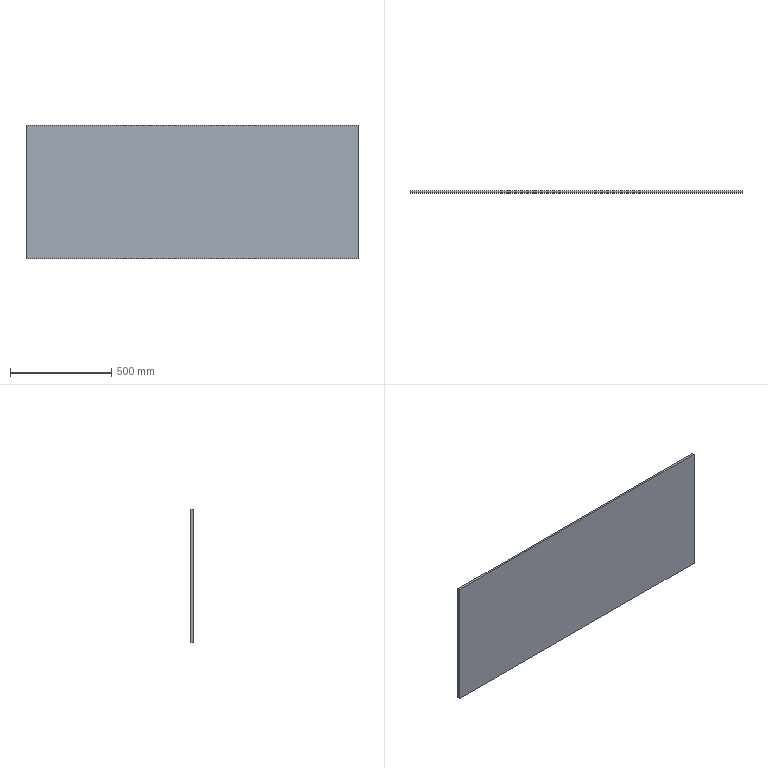Part | STEP file | zhichenban | 1 solid | 6 faces | box 1640 x 10 x 660 mm | volume 10824000 mm3 | plane 6
STEP:
#1=CARTESIAN_POINT('',(0.,0.,0.));
#2=DIRECTION('',(0.,0.,1.));
#3=DIRECTION('',(1.,0.,0.));
#4=AXIS2_PLACEMENT_3D('',#1,#2,#3);
#5=CARTESIAN_POINT('',(820.,0.,330.));
#6=VERTEX_POINT('',#5);
#7=CARTESIAN_POINT('',(820.,0.,-330.));
#8=VERTEX_POINT('',#7);
#9=CARTESIAN_POINT('',(820.,0.,-330.));
#10=DIRECTION('',(0.,0.,-1.));
#11=VECTOR('',#10,1.);
#12=LINE('',#9,#11);
#13=CARTESIAN_POINT('',(820.,10.,-330.));
#14=DIRECTION('',(-1.,0.,0.));
#15=DIRECTION('',(0.,0.,1.));
#16=AXIS2_PLACEMENT_3D('',#13,#14,#15);
#17=PLANE('',#16);
#18=CARTESIAN_POINT('',(0.,-10.));
#19=DIRECTION('',(-1.,0.));
#20=VECTOR('',#19,1.);
#21=LINE('',#18,#20);
#22=(GEOMETRIC_REPRESENTATION_CONTEXT(2)PARAMETRIC_REPRESENTATION_CONTEXT()REPRESENTATION_CONTEXT('',''));
#23=DEFINITIONAL_REPRESENTATION('',(#21),#22);
#24=PCURVE('',#17,#23);
#25=CARTESIAN_POINT('',(0.,0.,0.));
#26=DIRECTION('',(0.,1.,0.));
#27=DIRECTION('',(0.,0.,1.));
#28=AXIS2_PLACEMENT_3D('',#25,#26,#27);
#29=PLANE('',#28);
#30=CARTESIAN_POINT('',(-330.,820.));
#31=DIRECTION('',(-1.,0.));
#32=VECTOR('',#31,1.);
#33=LINE('',#30,#32);
#34=(GEOMETRIC_REPRESENTATION_CONTEXT(2)PARAMETRIC_REPRESENTATION_CONTEXT()REPRESENTATION_CONTEXT('',''));
#35=DEFINITIONAL_REPRESENTATION('',(#33),#34);
#36=PCURVE('',#29,#35);
#37=SURFACE_CURVE('',#12,(#24,#36),.PCURVE_S1.);
#38=EDGE_CURVE('',#6,#8,#37,.T.);
#39=ORIENTED_EDGE('',*,*,#38,.T.);
#40=CARTESIAN_POINT('',(820.,10.,-330.));
#41=VERTEX_POINT('',#40);
#42=CARTESIAN_POINT('',(820.,10.,-330.));
#43=DIRECTION('',(0.,-1.,0.));
#44=VECTOR('',#43,1.);
#45=LINE('',#42,#44);
#46=CARTESIAN_POINT('',(0.,0.));
#47=DIRECTION('',(0.,-1.));
#48=VECTOR('',#47,1.);
#49=LINE('',#46,#48);
#50=(GEOMETRIC_REPRESENTATION_CONTEXT(2)PARAMETRIC_REPRESENTATION_CONTEXT()REPRESENTATION_CONTEXT('',''));
#51=DEFINITIONAL_REPRESENTATION('',(#49),#50);
#52=PCURVE('',#17,#51);
#53=CARTESIAN_POINT('',(-820.,10.,-330.));
#54=DIRECTION('',(0.,0.,1.));
#55=DIRECTION('',(1.,0.,0.));
#56=AXIS2_PLACEMENT_3D('',#53,#54,#55);
#57=PLANE('',#56);
#58=CARTESIAN_POINT('',(1640.,0.));
#59=DIRECTION('',(0.,-1.));
#60=VECTOR('',#59,1.);
#61=LINE('',#58,#60);
#62=(GEOMETRIC_REPRESENTATION_CONTEXT(2)PARAMETRIC_REPRESENTATION_CONTEXT()REPRESENTATION_CONTEXT('',''));
#63=DEFINITIONAL_REPRESENTATION('',(#61),#62);
#64=PCURVE('',#57,#63);
#65=SURFACE_CURVE('',#45,(#52,#64),.PCURVE_S1.);
#66=EDGE_CURVE('',#41,#8,#65,.T.);
#67=ORIENTED_EDGE('',*,*,#66,.F.);
#68=CARTESIAN_POINT('',(820.,10.,330.));
#69=VERTEX_POINT('',#68);
#70=CARTESIAN_POINT('',(820.,10.,-330.));
#71=DIRECTION('',(0.,0.,-1.));
#72=VECTOR('',#71,1.);
#73=LINE('',#70,#72);
#74=CARTESIAN_POINT('',(0.,0.));
#75=DIRECTION('',(-1.,0.));
#76=VECTOR('',#75,1.);
#77=LINE('',#74,#76);
#78=(GEOMETRIC_REPRESENTATION_CONTEXT(2)PARAMETRIC_REPRESENTATION_CONTEXT()REPRESENTATION_CONTEXT('',''));
#79=DEFINITIONAL_REPRESENTATION('',(#77),#78);
#80=PCURVE('',#17,#79);
#81=CARTESIAN_POINT('',(0.,10.,0.));
#82=DIRECTION('',(0.,1.,0.));
#83=DIRECTION('',(0.,0.,1.));
#84=AXIS2_PLACEMENT_3D('',#81,#82,#83);
#85=PLANE('',#84);
#86=CARTESIAN_POINT('',(-330.,820.));
#87=DIRECTION('',(-1.,0.));
#88=VECTOR('',#87,1.);
#89=LINE('',#86,#88);
#90=(GEOMETRIC_REPRESENTATION_CONTEXT(2)PARAMETRIC_REPRESENTATION_CONTEXT()REPRESENTATION_CONTEXT('',''));
#91=DEFINITIONAL_REPRESENTATION('',(#89),#90);
#92=PCURVE('',#85,#91);
#93=SURFACE_CURVE('',#73,(#80,#92),.PCURVE_S1.);
#94=EDGE_CURVE('',#69,#41,#93,.T.);
#95=ORIENTED_EDGE('',*,*,#94,.F.);
#96=CARTESIAN_POINT('',(820.,10.,330.));
#97=DIRECTION('',(0.,-1.,0.));
#98=VECTOR('',#97,1.);
#99=LINE('',#96,#98);
#100=CARTESIAN_POINT('',(660.,0.));
#101=DIRECTION('',(0.,-1.));
#102=VECTOR('',#101,1.);
#103=LINE('',#100,#102);
#104=(GEOMETRIC_REPRESENTATION_CONTEXT(2)PARAMETRIC_REPRESENTATION_CONTEXT()REPRESENTATION_CONTEXT('',''));
#105=DEFINITIONAL_REPRESENTATION('',(#103),#104);
#106=PCURVE('',#17,#105);
#107=CARTESIAN_POINT('',(-820.,10.,330.));
#108=DIRECTION('',(0.,0.,-1.));
#109=DIRECTION('',(-1.,0.,0.));
#110=AXIS2_PLACEMENT_3D('',#107,#108,#109);
#111=PLANE('',#110);
#112=CARTESIAN_POINT('',(-1640.,0.));
#113=DIRECTION('',(0.,-1.));
#114=VECTOR('',#113,1.);
#115=LINE('',#112,#114);
#116=(GEOMETRIC_REPRESENTATION_CONTEXT(2)PARAMETRIC_REPRESENTATION_CONTEXT()REPRESENTATION_CONTEXT('',''));
#117=DEFINITIONAL_REPRESENTATION('',(#115),#116);
#118=PCURVE('',#111,#117);
#119=SURFACE_CURVE('',#99,(#106,#118),.PCURVE_S1.);
#120=EDGE_CURVE('',#69,#6,#119,.T.);
#121=ORIENTED_EDGE('',*,*,#120,.T.);
#122=EDGE_LOOP('',(#39,#67,#95,#121));
#123=FACE_BOUND('',#122,.T.);
#124=ADVANCED_FACE('',(#123),#17,.F.);
#125=CARTESIAN_POINT('',(-820.,0.,-330.));
#126=VERTEX_POINT('',#125);
#127=CARTESIAN_POINT('',(-820.,0.,-330.));
#128=DIRECTION('',(-1.,0.,0.));
#129=VECTOR('',#128,1.);
#130=LINE('',#127,#129);
#131=CARTESIAN_POINT('',(0.,-10.));
#132=DIRECTION('',(-1.,0.));
#133=VECTOR('',#132,1.);
#134=LINE('',#131,#133);
#135=(GEOMETRIC_REPRESENTATION_CONTEXT(2)PARAMETRIC_REPRESENTATION_CONTEXT()REPRESENTATION_CONTEXT('',''));
#136=DEFINITIONAL_REPRESENTATION('',(#134),#135);
#137=PCURVE('',#57,#136);
#138=CARTESIAN_POINT('',(-330.,-820.));
#139=DIRECTION('',(0.,-1.));
#140=VECTOR('',#139,1.);
#141=LINE('',#138,#140);
#142=(GEOMETRIC_REPRESENTATION_CONTEXT(2)PARAMETRIC_REPRESENTATION_CONTEXT()REPRESENTATION_CONTEXT('',''));
#143=DEFINITIONAL_REPRESENTATION('',(#141),#142);
#144=PCURVE('',#29,#143);
#145=SURFACE_CURVE('',#130,(#137,#144),.PCURVE_S1.);
#146=EDGE_CURVE('',#8,#126,#145,.T.);
#147=ORIENTED_EDGE('',*,*,#146,.T.);
#148=CARTESIAN_POINT('',(-820.,10.,-330.));
#149=VERTEX_POINT('',#148);
#150=CARTESIAN_POINT('',(-820.,10.,-330.));
#151=DIRECTION('',(0.,-1.,0.));
#152=VECTOR('',#151,1.);
#153=LINE('',#150,#152);
#154=CARTESIAN_POINT('',(0.,0.));
#155=DIRECTION('',(0.,-1.));
#156=VECTOR('',#155,1.);
#157=LINE('',#154,#156);
#158=(GEOMETRIC_REPRESENTATION_CONTEXT(2)PARAMETRIC_REPRESENTATION_CONTEXT()REPRESENTATION_CONTEXT('',''));
#159=DEFINITIONAL_REPRESENTATION('',(#157),#158);
#160=PCURVE('',#57,#159);
#161=CARTESIAN_POINT('',(-820.,10.,-330.));
#162=DIRECTION('',(1.,0.,0.));
#163=DIRECTION('',(0.,0.,-1.));
#164=AXIS2_PLACEMENT_3D('',#161,#162,#163);
#165=PLANE('',#164);
#166=CARTESIAN_POINT('',(0.,0.));
#167=DIRECTION('',(0.,-1.));
#168=VECTOR('',#167,1.);
#169=LINE('',#166,#168);
#170=(GEOMETRIC_REPRESENTATION_CONTEXT(2)PARAMETRIC_REPRESENTATION_CONTEXT()REPRESENTATION_CONTEXT('',''));
#171=DEFINITIONAL_REPRESENTATION('',(#169),#170);
#172=PCURVE('',#165,#171);
#173=SURFACE_CURVE('',#153,(#160,#172),.PCURVE_S1.);
#174=EDGE_CURVE('',#149,#126,#173,.T.);
#175=ORIENTED_EDGE('',*,*,#174,.F.);
#176=CARTESIAN_POINT('',(-820.,10.,-330.));
#177=DIRECTION('',(-1.,0.,0.));
#178=VECTOR('',#177,1.);
#179=LINE('',#176,#178);
#180=CARTESIAN_POINT('',(0.,0.));
#181=DIRECTION('',(-1.,0.));
#182=VECTOR('',#181,1.);
#183=LINE('',#180,#182);
#184=(GEOMETRIC_REPRESENTATION_CONTEXT(2)PARAMETRIC_REPRESENTATION_CONTEXT()REPRESENTATION_CONTEXT('',''));
#185=DEFINITIONAL_REPRESENTATION('',(#183),#184);
#186=PCURVE('',#57,#185);
#187=CARTESIAN_POINT('',(-330.,-820.));
#188=DIRECTION('',(0.,-1.));
#189=VECTOR('',#188,1.);
#190=LINE('',#187,#189);
#191=(GEOMETRIC_REPRESENTATION_CONTEXT(2)PARAMETRIC_REPRESENTATION_CONTEXT()REPRESENTATION_CONTEXT('',''));
#192=DEFINITIONAL_REPRESENTATION('',(#190),#191);
#193=PCURVE('',#85,#192);
#194=SURFACE_CURVE('',#179,(#186,#193),.PCURVE_S1.);
#195=EDGE_CURVE('',#41,#149,#194,.T.);
#196=ORIENTED_EDGE('',*,*,#195,.F.);
#197=ORIENTED_EDGE('',*,*,#66,.T.);
#198=EDGE_LOOP('',(#147,#175,#196,#197));
#199=FACE_BOUND('',#198,.T.);
#200=ADVANCED_FACE('',(#199),#57,.F.);
#201=CARTESIAN_POINT('',(-820.,0.,330.));
#202=VERTEX_POINT('',#201);
#203=CARTESIAN_POINT('',(-820.,0.,-330.));
#204=DIRECTION('',(0.,0.,1.));
#205=VECTOR('',#204,1.);
#206=LINE('',#203,#205);
#207=CARTESIAN_POINT('',(0.,-10.));
#208=DIRECTION('',(-1.,0.));
#209=VECTOR('',#208,1.);
#210=LINE('',#207,#209);
#211=(GEOMETRIC_REPRESENTATION_CONTEXT(2)PARAMETRIC_REPRESENTATION_CONTEXT()REPRESENTATION_CONTEXT('',''));
#212=DEFINITIONAL_REPRESENTATION('',(#210),#211);
#213=PCURVE('',#165,#212);
#214=CARTESIAN_POINT('',(-330.,-820.));
#215=DIRECTION('',(1.,0.));
#216=VECTOR('',#215,1.);
#217=LINE('',#214,#216);
#218=(GEOMETRIC_REPRESENTATION_CONTEXT(2)PARAMETRIC_REPRESENTATION_CONTEXT()REPRESENTATION_CONTEXT('',''));
#219=DEFINITIONAL_REPRESENTATION('',(#217),#218);
#220=PCURVE('',#29,#219);
#221=SURFACE_CURVE('',#206,(#213,#220),.PCURVE_S1.);
#222=EDGE_CURVE('',#126,#202,#221,.T.);
#223=ORIENTED_EDGE('',*,*,#222,.T.);
#224=CARTESIAN_POINT('',(-820.,10.,330.));
#225=VERTEX_POINT('',#224);
#226=CARTESIAN_POINT('',(-820.,10.,330.));
#227=DIRECTION('',(0.,-1.,0.));
#228=VECTOR('',#227,1.);
#229=LINE('',#226,#228);
#230=CARTESIAN_POINT('',(-660.,0.));
#231=DIRECTION('',(0.,-1.));
#232=VECTOR('',#231,1.);
#233=LINE('',#230,#232);
#234=(GEOMETRIC_REPRESENTATION_CONTEXT(2)PARAMETRIC_REPRESENTATION_CONTEXT()REPRESENTATION_CONTEXT('',''));
#235=DEFINITIONAL_REPRESENTATION('',(#233),#234);
#236=PCURVE('',#165,#235);
#237=CARTESIAN_POINT('',(0.,0.));
#238=DIRECTION('',(0.,-1.));
#239=VECTOR('',#238,1.);
#240=LINE('',#237,#239);
#241=(GEOMETRIC_REPRESENTATION_CONTEXT(2)PARAMETRIC_REPRESENTATION_CONTEXT()REPRESENTATION_CONTEXT('',''));
#242=DEFINITIONAL_REPRESENTATION('',(#240),#241);
#243=PCURVE('',#111,#242);
#244=SURFACE_CURVE('',#229,(#236,#243),.PCURVE_S1.);
#245=EDGE_CURVE('',#225,#202,#244,.T.);
#246=ORIENTED_EDGE('',*,*,#245,.F.);
#247=CARTESIAN_POINT('',(-820.,10.,-330.));
#248=DIRECTION('',(0.,0.,1.));
#249=VECTOR('',#248,1.);
#250=LINE('',#247,#249);
#251=CARTESIAN_POINT('',(0.,0.));
#252=DIRECTION('',(-1.,0.));
#253=VECTOR('',#252,1.);
#254=LINE('',#251,#253);
#255=(GEOMETRIC_REPRESENTATION_CONTEXT(2)PARAMETRIC_REPRESENTATION_CONTEXT()REPRESENTATION_CONTEXT('',''));
#256=DEFINITIONAL_REPRESENTATION('',(#254),#255);
#257=PCURVE('',#165,#256);
#258=CARTESIAN_POINT('',(-330.,-820.));
#259=DIRECTION('',(1.,0.));
#260=VECTOR('',#259,1.);
#261=LINE('',#258,#260);
#262=(GEOMETRIC_REPRESENTATION_CONTEXT(2)PARAMETRIC_REPRESENTATION_CONTEXT()REPRESENTATION_CONTEXT('',''));
#263=DEFINITIONAL_REPRESENTATION('',(#261),#262);
#264=PCURVE('',#85,#263);
#265=SURFACE_CURVE('',#250,(#257,#264),.PCURVE_S1.);
#266=EDGE_CURVE('',#149,#225,#265,.T.);
#267=ORIENTED_EDGE('',*,*,#266,.F.);
#268=ORIENTED_EDGE('',*,*,#174,.T.);
#269=EDGE_LOOP('',(#223,#246,#267,#268));
#270=FACE_BOUND('',#269,.T.);
#271=ADVANCED_FACE('',(#270),#165,.F.);
#272=CARTESIAN_POINT('',(-820.,0.,330.));
#273=DIRECTION('',(1.,0.,0.));
#274=VECTOR('',#273,1.);
#275=LINE('',#272,#274);
#276=CARTESIAN_POINT('',(0.,-10.));
#277=DIRECTION('',(-1.,0.));
#278=VECTOR('',#277,1.);
#279=LINE('',#276,#278);
#280=(GEOMETRIC_REPRESENTATION_CONTEXT(2)PARAMETRIC_REPRESENTATION_CONTEXT()REPRESENTATION_CONTEXT('',''));
#281=DEFINITIONAL_REPRESENTATION('',(#279),#280);
#282=PCURVE('',#111,#281);
#283=CARTESIAN_POINT('',(330.,-820.));
#284=DIRECTION('',(0.,1.));
#285=VECTOR('',#284,1.);
#286=LINE('',#283,#285);
#287=(GEOMETRIC_REPRESENTATION_CONTEXT(2)PARAMETRIC_REPRESENTATION_CONTEXT()REPRESENTATION_CONTEXT('',''));
#288=DEFINITIONAL_REPRESENTATION('',(#286),#287);
#289=PCURVE('',#29,#288);
#290=SURFACE_CURVE('',#275,(#282,#289),.PCURVE_S1.);
#291=EDGE_CURVE('',#202,#6,#290,.T.);
#292=ORIENTED_EDGE('',*,*,#291,.T.);
#293=ORIENTED_EDGE('',*,*,#120,.F.);
#294=CARTESIAN_POINT('',(-820.,10.,330.));
#295=DIRECTION('',(1.,0.,0.));
#296=VECTOR('',#295,1.);
#297=LINE('',#294,#296);
#298=CARTESIAN_POINT('',(0.,0.));
#299=DIRECTION('',(-1.,0.));
#300=VECTOR('',#299,1.);
#301=LINE('',#298,#300);
#302=(GEOMETRIC_REPRESENTATION_CONTEXT(2)PARAMETRIC_REPRESENTATION_CONTEXT()REPRESENTATION_CONTEXT('',''));
#303=DEFINITIONAL_REPRESENTATION('',(#301),#302);
#304=PCURVE('',#111,#303);
#305=CARTESIAN_POINT('',(330.,-820.));
#306=DIRECTION('',(0.,1.));
#307=VECTOR('',#306,1.);
#308=LINE('',#305,#307);
#309=(GEOMETRIC_REPRESENTATION_CONTEXT(2)PARAMETRIC_REPRESENTATION_CONTEXT()REPRESENTATION_CONTEXT('',''));
#310=DEFINITIONAL_REPRESENTATION('',(#308),#309);
#311=PCURVE('',#85,#310);
#312=SURFACE_CURVE('',#297,(#304,#311),.PCURVE_S1.);
#313=EDGE_CURVE('',#225,#69,#312,.T.);
#314=ORIENTED_EDGE('',*,*,#313,.F.);
#315=ORIENTED_EDGE('',*,*,#245,.T.);
#316=EDGE_LOOP('',(#292,#293,#314,#315));
#317=FACE_BOUND('',#316,.T.);
#318=ADVANCED_FACE('',(#317),#111,.F.);
#319=ORIENTED_EDGE('',*,*,#94,.T.);
#320=ORIENTED_EDGE('',*,*,#195,.T.);
#321=ORIENTED_EDGE('',*,*,#266,.T.);
#322=ORIENTED_EDGE('',*,*,#313,.T.);
#323=EDGE_LOOP('',(#319,#320,#321,#322));
#324=FACE_BOUND('',#323,.T.);
#325=ADVANCED_FACE('',(#324),#85,.T.);
#326=ORIENTED_EDGE('',*,*,#38,.F.);
#327=ORIENTED_EDGE('',*,*,#291,.F.);
#328=ORIENTED_EDGE('',*,*,#222,.F.);
#329=ORIENTED_EDGE('',*,*,#146,.F.);
#330=EDGE_LOOP('',(#326,#327,#328,#329));
#331=FACE_BOUND('',#330,.T.);
#332=ADVANCED_FACE('',(#331),#29,.F.);
#333=CLOSED_SHELL('',(#124,#200,#271,#318,#325,#332));
#334=MANIFOLD_SOLID_BREP('',#333);
#335=(LENGTH_UNIT()NAMED_UNIT(*)SI_UNIT(.MILLI.,.METRE.));
#336=UNCERTAINTY_MEASURE_WITH_UNIT(LENGTH_MEASURE(0.0000001),#335,'','');
#337=(NAMED_UNIT(*)PLANE_ANGLE_UNIT()SI_UNIT($,.RADIAN.));
#338=(NAMED_UNIT(*)SI_UNIT($,.STERADIAN.)SOLID_ANGLE_UNIT());
#339=(GEOMETRIC_REPRESENTATION_CONTEXT(3)GLOBAL_UNCERTAINTY_ASSIGNED_CONTEXT((#336))GLOBAL_UNIT_ASSIGNED_CONTEXT((#335,#337,#338))REPRESENTATION_CONTEXT('',''));
#340=ADVANCED_BREP_SHAPE_REPRESENTATION('',(#4,#334),#339);